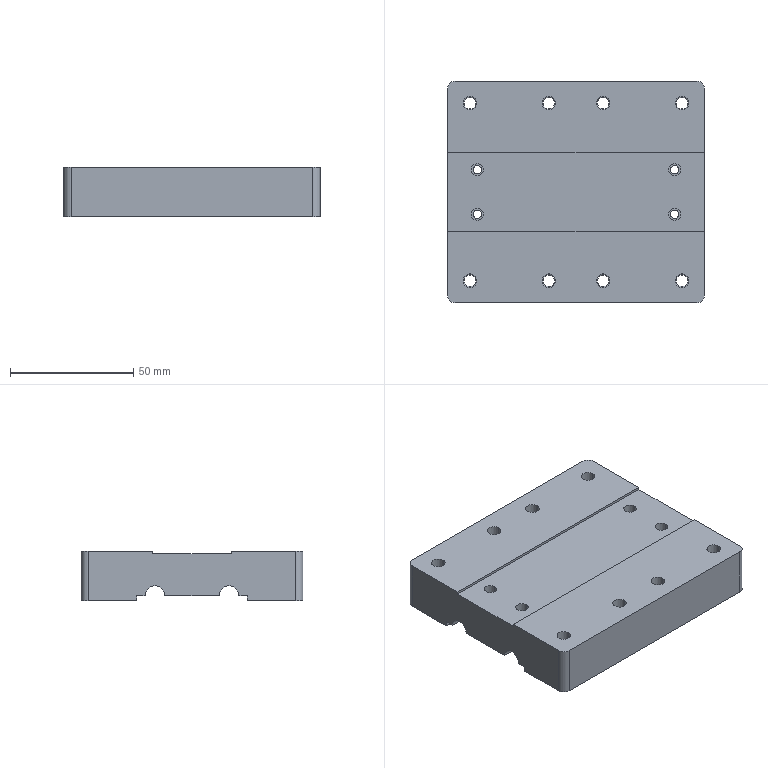Part | STEP file | MJ45 slider | 1 solid | 76 faces | box 104 x 90 x 20 mm | volume 164549 mm3 | cylinder 40 | plane 20 | cone 16 | commonest cylinder face diameters 5.5 x16 3.4 x8 5 x8 6 x4 8 x4